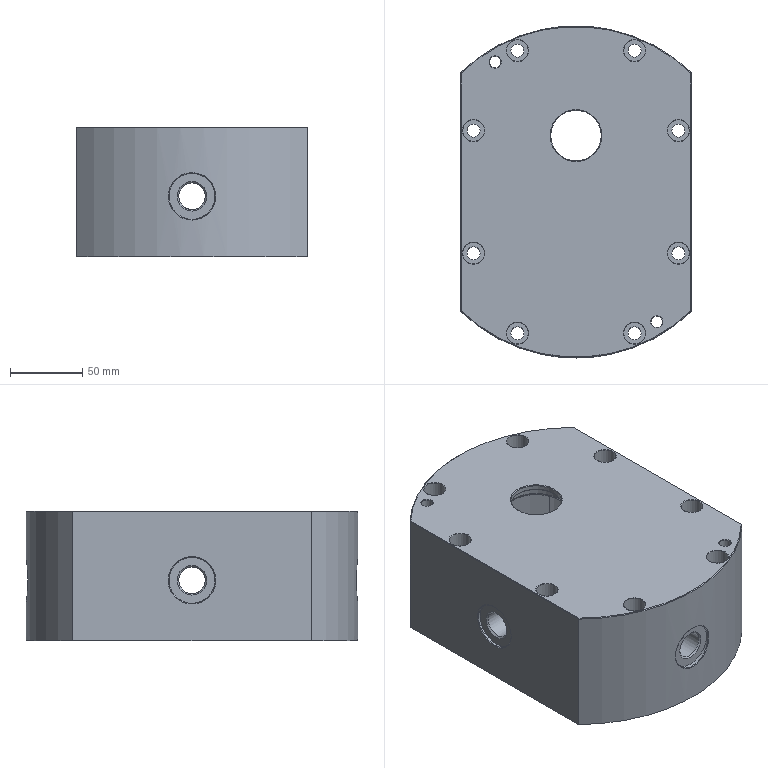NC program | NX | posted with a generic post | part box 160 x 230 x 90 mm
Lines 1 to 991 of 9223:
N10 G17 G21 G94 G90
(FLOOR_WALL_COPY_1 , TOOL : D50)
N12 T02 M6
N14 G54
N16 G17 G0 G90 X-153. Y89.997 B0. C0. S1200 M3
N18 G43 Z30. H2
N20 Z12.658
N22 G94 G1 Z9.658 F1000.
N24 X-150.
N26 X150. F2000.
N28 Y49.998
N30 X-150.
N32 Y9.999
N34 X150.
N36 Y-30.001
N38 X-150.
N40 Y-65.341
N42 Y-70.
N44 X150.
N46 X153.
N48 Z12.658
N50 G0 Z30.
N52 X-153. Y89.997
N54 Z12.317
N56 G1 Z9.317 F1000.
N58 X-150.
N60 X150. F2000.
N62 Y49.998
N64 X-150.
N66 Y9.999
N68 X150.
N70 Y-30.001
N72 X-150.
N74 Y-65.341
N76 Y-70.
N78 X150.
N80 X153.
N82 Z12.317
N84 G0 Z30.
N86 X-153. Y89.997
N88 Z11.976
N90 G1 Z8.976 F1000.
N92 X-150.
N94 X150. F2000.
N96 Y49.998
N98 X-150.
N100 Y9.999
N102 X150.
N104 Y-30.001
N106 X-150.
N108 Y-65.341
N110 Y-70.
N112 X150.
N114 X153.
N116 Z11.976
N118 G0 Z30.
N120 X-153. Y89.997
N122 Z11.634
N124 G1 Z8.634 F1000.
N126 X-150.
N128 X150. F2000.
N130 Y49.998
N132 X-150.
N134 Y9.999
N136 X150.
N138 Y-30.001
N140 X-150.
N142 Y-65.341
N144 Y-70.
N146 X150.
N148 X153.
N150 Z11.634
N152 G0 Z30.
N154 X-153. Y89.997
N156 Z11.293
N158 G1 Z8.293 F1000.
N160 X-150.
N162 X150. F2000.
N164 Y49.998
N166 X-150.
N168 Y9.999
N170 X150.
N172 Y-30.001
N174 X-150.
N176 Y-65.341
N178 Y-70.
N180 X150.
N182 X153.
N184 Z11.293
N186 G0 Z30.
N188 X-153. Y89.997
N190 Z10.951
N192 G1 Z7.951 F1000.
N194 X-150.
N196 X150. F2000.
N198 Y49.998
N200 X-150.
N202 Y9.999
N204 X150.
N206 Y-30.001
N208 X-150.
N210 Y-65.341
N212 Y-70.
N214 X150.
N216 X153.
N218 Z10.951
N220 G0 Z30.
N222 X-153. Y89.997
N224 Z10.61
N226 G1 Z7.61 F1000.
N228 X-150.
N230 X150. F2000.
N232 Y49.998
N234 X-150.
N236 Y9.999
N238 X150.
N240 Y-30.001
N242 X-150.
N244 Y-65.341
N246 Y-70.
N248 X150.
N250 X153.
N252 Z10.61
N254 G0 Z30.
N256 X-153. Y89.997
N258 Z10.269
N260 G1 Z7.269 F1000.
N262 X-150.
N264 X150. F2000.
N266 Y49.998
N268 X-150.
N270 Y9.999
N272 X150.
N274 Y-30.001
N276 X-150.
N278 Y-65.341
N280 Y-70.
N282 X150.
N284 X153.
N286 Z10.269
N288 G0 Z30.
N290 X-153. Y89.997
N292 Z9.927
N294 G1 Z6.927 F1000.
N296 X-150.
N298 X150. F2000.
N300 Y49.998
N302 X-150.
N304 Y9.999
N306 X150.
N308 Y-30.001
N310 X-150.
N312 Y-65.341
N314 Y-70.
N316 X150.
N318 X153.
N320 Z9.927
N322 G0 Z30.
N324 X-153. Y89.997
N326 Z9.586
N328 G1 Z6.586 F1000.
N330 X-150.
N332 X150. F2000.
N334 Y49.998
N336 X-150.
N338 Y9.999
N340 X150.
N342 Y-30.001
N344 X-150.
N346 Y-65.341
N348 Y-70.
N350 X150.
N352 X153.
N354 Z9.586
N356 G0 Z30.
N358 X-153. Y89.997
N360 Z9.245
N362 G1 Z6.245 F1000.
N364 X-150.
N366 X150. F2000.
N368 Y49.998
N370 X-150.
N372 Y9.999
N374 X150.
N376 Y-30.001
N378 X-150.
N380 Y-65.341
N382 Y-70.
N384 X150.
N386 X153.
N388 Z9.245
N390 G0 Z30.
N392 X-153. Y89.997
N394 Z8.903
N396 G1 Z5.903 F1000.
N398 X-150.
N400 X150. F2000.
N402 Y49.998
N404 X-150.
N406 Y9.999
N408 X150.
N410 Y-30.001
N412 X-150.
N414 Y-65.341
N416 Y-70.
N418 X150.
N420 X153.
N422 Z8.903
N424 G0 Z30.
N426 X-153. Y89.997
N428 Z8.562
N430 G1 Z5.562 F1000.
N432 X-150.
N434 X150. F2000.
N436 Y49.998
N438 X-150.
N440 Y9.999
N442 X150.
N444 Y-30.001
N446 X-150.
N448 Y-65.341
N450 Y-70.
N452 X150.
N454 X153.
N456 Z8.562
N458 G0 Z30.
N460 X-153. Y89.997
N462 Z8.221
N464 G1 Z5.221 F1000.
N466 X-150.
N468 X150. F2000.
N470 Y49.998
N472 X-150.
N474 Y9.999
N476 X150.
N478 Y-30.001
N480 X-150.
N482 Y-65.341
N484 Y-70.
N486 X150.
N488 X153.
N490 Z8.221
N492 G0 Z30.
N494 X-153. Y89.997
N496 Z7.879
N498 G1 Z4.879 F1000.
N500 X-150.
N502 X150. F2000.
N504 Y49.998
N506 X-150.
N508 Y9.999
N510 X150.
N512 Y-30.001
N514 X-150.
N516 Y-65.341
N518 Y-70.
N520 X150.
N522 X153.
N524 Z7.879
N526 G0 Z30.
N528 X-153. Y89.997
N530 Z7.538
N532 G1 Z4.538 F1000.
N534 X-150.
N536 X150. F2000.
N538 Y49.998
N540 X-150.
N542 Y9.999
N544 X150.
N546 Y-30.001
N548 X-150.
N550 Y-65.341
N552 Y-70.
N554 X150.
N556 X153.
N558 Z7.538
N560 G0 Z30.
N562 X-153. Y89.997
N564 Z7.196
N566 G1 Z4.196 F1000.
N568 X-150.
N570 X150. F2000.
N572 Y49.998
N574 X-150.
N576 Y9.999
N578 X150.
N580 Y-30.001
N582 X-150.
N584 Y-65.341
N586 Y-70.
N588 X150.
N590 X153.
N592 Z7.196
N594 G0 Z30.
N596 X-153. Y89.997
N598 Z6.855
N600 G1 Z3.855 F1000.
N602 X-150.
N604 X150. F2000.
N606 Y49.998
N608 X-150.
N610 Y9.999
N612 X150.
N614 Y-30.001
N616 X-150.
N618 Y-65.341
N620 Y-70.
N622 X150.
N624 X153.
N626 Z6.855
N628 G0 Z30.
N630 X-153. Y89.997
N632 Z6.514
N634 G1 Z3.514 F1000.
N636 X-150.
N638 X150. F2000.
N640 Y49.998
N642 X-150.
N644 Y9.999
N646 X150.
N648 Y-30.001
N650 X-150.
N652 Y-65.341
N654 Y-70.
N656 X150.
N658 X153.
N660 Z6.514
N662 G0 Z30.
N664 X-153. Y89.997
N666 Z6.172
N668 G1 Z3.172 F1000.
N670 X-150.
N672 X150. F2000.
N674 Y49.998
N676 X-150.
N678 Y9.999
N680 X150.
N682 Y-30.001
N684 X-150.
N686 Y-65.341
N688 Y-70.
N690 X150.
N692 X153.
N694 Z6.172
N696 G0 Z30.
N698 X-153. Y89.997
N700 Z5.831
N702 G1 Z2.831 F1000.
N704 X-150.
N706 X150. F2000.
N708 Y49.998
N710 X-150.
N712 Y9.999
N714 X150.
N716 Y-30.001
N718 X-150.
N720 Y-65.341
N722 Y-70.
N724 X150.
N726 X153.
N728 Z5.831
N730 G0 Z30.
N732 X-153. Y89.997
N734 Z5.49
N736 G1 Z2.49 F1000.
N738 X-150.
N740 X150. F2000.
N742 Y49.998
N744 X-150.
N746 Y9.999
N748 X150.
N750 Y-30.001
N752 X-150.
N754 Y-65.341
N756 Y-70.
N758 X150.
N760 X153.
N762 Z5.49
N764 G0 Z30.
N766 X-153. Y89.997
N768 Z5.148
N770 G1 Z2.148 F1000.
N772 X-150.
N774 X150. F2000.
N776 Y49.998
N778 X-150.
N780 Y9.999
N782 X150.
N784 Y-30.001
N786 X-150.
N788 Y-65.341
N790 Y-70.
N792 X150.
N794 X153.
N796 Z5.148
N798 G0 Z30.
N800 X-153. Y89.997
N802 Z4.807
N804 G1 Z1.807 F1000.
N806 X-150.
N808 X150. F2000.
N810 Y49.998
N812 X-150.
N814 Y9.999
N816 X150.
N818 Y-30.001
N820 X-150.
N822 Y-65.341
N824 Y-70.
N826 X150.
N828 X153.
N830 Z4.807
N832 G0 Z30.
N834 X-153. Y89.997
N836 Z4.465
N838 G1 Z1.465 F1000.
N840 X-150.
N842 X150. F2000.
N844 Y49.998
N846 X-150.
N848 Y9.999
N850 X150.
N852 Y-30.001
N854 X-150.
N856 Y-65.341
N858 Y-70.
N860 X150.
N862 X153.
N864 Z4.465
N866 G0 Z30.
N868 X-153. Y89.997
N870 Z4.124
N872 G1 Z1.124 F1000.
N874 X-150.
N876 X150. F2000.
N878 Y49.998
N880 X-150.
N882 Y9.999
N884 X150.
N886 Y-30.001
N888 X-150.
N890 Y-65.341
N892 Y-70.
N894 X150.
N896 X153.
N898 Z4.124
N900 G0 Z30.
N902 X-153. Y89.997
N904 Z3.783
N906 G1 Z0.783 F1000.
N908 X-150.
N910 X150. F2000.
N912 Y49.998
N914 X-150.
N916 Y9.999
N918 X150.
N920 Y-30.001
N922 X-150.
N924 Y-65.341
N926 Y-70.
N928 X150.
N930 X153.
N932 Z3.783
N934 G0 Z30.
N936 X-153. Y89.997
N938 Z3.441
N940 G1 Z0.441 F1000.
N942 X-150.
N944 X150. F2000.
N946 Y49.998
N948 X-150.
N950 Y9.999
N952 X150.
N954 Y-30.001
N956 X-150.
N958 Y-65.341
N960 Y-70.
N962 X150.
N964 X153.
N966 Z3.441
N968 G0 Z30.
N970 X-153. Y89.997
N972 Z3.1
N974 G1 Z0.1 F1000.
N976 X-150.
N978 X150. F2000.
N980 Y49.998
N982 X-150.
N984 Y9.999
N986 X150.
N988 Y-30.001
N990 X-150.
N992 Y-65.341
N994 Y-70.
N996 X150.
N998 X153.
N1000 Z3.1
N1002 G0 Z30.
(FLOOR_WALL_COPY_COPY , TOOL : D50)
N1004 X-153. Y89.997 S2500
N1006 Z3.
N1008 G1 Z0. F1000.
N1010 X-150.
N1012 X150.
N1014 Y49.998
N1016 X-150.
N1018 Y9.999
N1020 X150.
N1022 Y-30.001
N1024 X-150.
N1026 Y-65.341
N1028 Y-70.
N1030 X150.
N1032 X153.
N1034 Z3.
N1036 G0 Z30.
N1038 M5
(DRILLING_COPY_1 , TOOL : ZXZ)
N1040 T01 M6
N1042 G54
N1044 G17 G0 G90 X-42.5 Y71. B0. C0. S5000 M3
N1046 G43 Z30. H1
N1048 G94 G81 G98 Z-1. F250. R3.
N1050 X-90. Y56.
N1052 X-97.931 Y40.564
N1054 Y-40.564
N1056 X-42.5 Y-71.
N1058 X42.5
N1060 X90. Y-56.
N1062 X97.931 Y-40.564
N1064 Y40.564
N1066 X42.5 Y71.
N1068 G80
N1070 G0 X42.5 Y71. Z30.
N1072 M5
(DRILLING_COPY , TOOL : 9.0ZT)
N1074 T09 M6
N1076 G54
N1078 G17 G0 G90 X42.5 Y-71. B0. C0. S2000 M3
N1080 G43 Z30. H9
N1082 G94 G83 G98 Z-69.204 F150. Q2. R3.
N1084 X97.931 Y-40.564
N1086 Y40.564
N1088 X42.5 Y71.
N1090 X-42.5
N1092 X-97.931 Y40.564
N1094 Y-40.564
N1096 X-42.5 Y-71.
N1098 G80
N1100 G0 X-42.5 Y-71. Z30.
N1102 M5
(DRILLING_COPY_COPY , TOOL : 7.8ZT)
N1104 T08 M6
N1106 G54
N1108 G17 G0 G90 X-90. Y56. B0. C0. S2000 M3
N1110 G43 Z30. H8
N1112 G94 G83 G98 Z-23.343 F150. Q2. R3.
N1114 X90. Y-56.
N1116 G80
N1118 G0 X90. Y-56. Z30.
N1120 M5
(DRILLING_COPY_COPY_COPY , TOOL : 8.0JD)
N1122 T18 M6
N1124 G54
N1126 G17 G0 G90 X-90. Y56. B0. C0. S800 M3
N1128 G43 Z30. H18
N1130 G94 G85 G98 Z-20. F40. R3.
N1132 X90. Y-56.
N1134 G80
N1136 G0 X90. Y-56. Z30.
N1138 M5
(PLANAR_PROFILE , TOOL : D3)
N1140 T03 M6
N1142 G54
N1144 G17 G0 G90 X0. Y62.5 B0. C0. S5000 M3
N1146 G43 Z30. H3
N1148 Z3.
N1150 G94 G1 Z-0.05 F500.
N1152 X-65.077 F1100.
N1154 G3 X-81.346 Y53.75 R19.5
N1156 X-81.346 Y-53.75 R97.5
N1158 X-65.077 Y-62.5 R19.5
N1160 G1 X65.077
N1162 G3 X81.346 Y-53.75 R19.5
N1164 X81.346 Y53.75 R97.5
N1166 X65.077 Y62.5 R19.5
N1168 G1 X0.
N1170 Z2.95
N1172 Z-0.1 F500.
N1174 X65.077 F1100.
N1176 G2 X81.346 Y53.75 R19.5
N1178 X81.346 Y-53.75 R97.5
N1180 X65.077 Y-62.5 R19.5
N1182 G1 X-65.077
N1184 G2 X-81.346 Y-53.75 R19.5
N1186 X-81.346 Y53.75 R97.5
N1188 X-65.077 Y62.5 R19.5
N1190 G1 X0.
N1192 Z2.9
N1194 Z-0.15 F500.
N1196 X-65.077 F1100.
N1198 G3 X-81.346 Y53.75 R19.5
N1200 X-81.346 Y-53.75 R97.5
N1202 X-65.077 Y-62.5 R19.5
N1204 G1 X65.077
N1206 G3 X81.346 Y-53.75 R19.5
N1208 X81.346 Y53.75 R97.5
N1210 X65.077 Y62.5 R19.5
N1212 G1 X0.
N1214 Z2.85
N1216 Z-0.2 F500.
N1218 X65.077 F1100.
N1220 G2 X81.346 Y53.75 R19.5
N1222 X81.346 Y-53.75 R97.5
N1224 X65.077 Y-62.5 R19.5
N1226 G1 X-65.077
N1228 G2 X-81.346 Y-53.75 R19.5
N1230 X-81.346 Y53.75 R97.5
N1232 X-65.077 Y62.5 R19.5
N1234 G1 X0.
N1236 Z2.8
N1238 Z-0.25 F500.
N1240 X-65.077 F1100.
N1242 G3 X-81.346 Y53.75 R19.5
N1244 X-81.346 Y-53.75 R97.5
N1246 X-65.077 Y-62.5 R19.5
N1248 G1 X65.077
N1250 G3 X81.346 Y-53.75 R19.5
N1252 X81.346 Y53.75 R97.5
N1254 X65.077 Y62.5 R19.5
N1256 G1 X0.
N1258 Z2.75
N1260 Z-0.3 F500.
N1262 X65.077 F1100.
N1264 G2 X81.346 Y53.75 R19.5
N1266 X81.346 Y-53.75 R97.5
N1268 X65.077 Y-62.5 R19.5
N1270 G1 X-65.077
N1272 G2 X-81.346 Y-53.75 R19.5
N1274 X-81.346 Y53.75 R97.5
N1276 X-65.077 Y62.5 R19.5
N1278 G1 X0.
N1280 Z2.7
N1282 Z-0.35 F500.
N1284 X-65.077 F1100.
N1286 G3 X-81.346 Y53.75 R19.5
N1288 X-81.346 Y-53.75 R97.5
N1290 X-65.077 Y-62.5 R19.5
N1292 G1 X65.077
N1294 G3 X81.346 Y-53.75 R19.5
N1296 X81.346 Y53.75 R97.5
N1298 X65.077 Y62.5 R19.5
N1300 G1 X0.
N1302 Z2.65
N1304 Z-0.4 F500.
N1306 X65.077 F1100.
N1308 G2 X81.346 Y53.75 R19.5
N1310 X81.346 Y-53.75 R97.5
N1312 X65.077 Y-62.5 R19.5
N1314 G1 X-65.077
N1316 G2 X-81.346 Y-53.75 R19.5
N1318 X-81.346 Y53.75 R97.5
N1320 X-65.077 Y62.5 R19.5
N1322 G1 X0.
N1324 Z2.6
N1326 Z-0.45 F500.
N1328 X-65.077 F1100.
N1330 G3 X-81.346 Y53.75 R19.5
N1332 X-81.346 Y-53.75 R97.5
N1334 X-65.077 Y-62.5 R19.5
N1336 G1 X65.077
N1338 G3 X81.346 Y-53.75 R19.5
N1340 X81.346 Y53.75 R97.5
N1342 X65.077 Y62.5 R19.5
N1344 G1 X0.
N1346 Z2.55
N1348 Z-0.5 F500.
N1350 X65.077 F1100.
N1352 G2 X81.346 Y53.75 R19.5
N1354 X81.346 Y-53.75 R97.5
N1356 X65.077 Y-62.5 R19.5
N1358 G1 X-65.077
N1360 G2 X-81.346 Y-53.75 R19.5
N1362 X-81.346 Y53.75 R97.5
N1364 X-65.077 Y62.5 R19.5
N1366 G1 X0.
N1368 Z2.5
N1370 Z-0.55 F500.
N1372 X-65.077 F1100.
N1374 G3 X-81.346 Y53.75 R19.5
N1376 X-81.346 Y-53.75 R97.5
N1378 X-65.077 Y-62.5 R19.5
N1380 G1 X65.077
N1382 G3 X81.346 Y-53.75 R19.5
N1384 X81.346 Y53.75 R97.5
N1386 X65.077 Y62.5 R19.5
N1388 G1 X0.
N1390 Z2.45
N1392 Z-0.6 F500.
N1394 X65.077 F1100.
N1396 G2 X81.346 Y53.75 R19.5
N1398 X81.346 Y-53.75 R97.5
N1400 X65.077 Y-62.5 R19.5
N1402 G1 X-65.077
N1404 G2 X-81.346 Y-53.75 R19.5
N1406 X-81.346 Y53.75 R97.5
N1408 X-65.077 Y62.5 R19.5
N1410 G1 X0.
N1412 Z2.4
N1414 Z-0.65 F500.
N1416 X-65.077 F1100.
N1418 G3 X-81.346 Y53.75 R19.5
N1420 X-81.346 Y-53.75 R97.5
N1422 X-65.077 Y-62.5 R19.5
N1424 G1 X65.077
N1426 G3 X81.346 Y-53.75 R19.5
N1428 X81.346 Y53.75 R97.5
N1430 X65.077 Y62.5 R19.5
N1432 G1 X0.
N1434 Z2.35
N1436 Z-0.7 F500.
N1438 X65.077 F1100.
N1440 G2 X81.346 Y53.75 R19.5
N1442 X81.346 Y-53.75 R97.5
N1444 X65.077 Y-62.5 R19.5
N1446 G1 X-65.077
N1448 G2 X-81.346 Y-53.75 R19.5
N1450 X-81.346 Y53.75 R97.5
N1452 X-65.077 Y62.5 R19.5
N1454 G1 X0.
N1456 Z2.3
N1458 Z-0.75 F500.
N1460 X-65.077 F1100.
N1462 G3 X-81.346 Y53.75 R19.5
N1464 X-81.346 Y-53.75 R97.5
N1466 X-65.077 Y-62.5 R19.5
N1468 G1 X65.077
N1470 G3 X81.346 Y-53.75 R19.5
N1472 X81.346 Y53.75 R97.5
N1474 X65.077 Y62.5 R19.5
N1476 G1 X0.
N1478 Z2.25
N1480 Z-0.8 F500.
N1482 X65.077 F1100.
N1484 G2 X81.346 Y53.75 R19.5
N1486 X81.346 Y-53.75 R97.5
N1488 X65.077 Y-62.5 R19.5
N1490 G1 X-65.077
N1492 G2 X-81.346 Y-53.75 R19.5
N1494 X-81.346 Y53.75 R97.5
N1496 X-65.077 Y62.5 R19.5
N1498 G1 X0.
N1500 Z2.2
N1502 Z-0.85 F500.
N1504 X-65.077 F1100.
N1506 G3 X-81.346 Y53.75 R19.5
N1508 X-81.346 Y-53.75 R97.5
N1510 X-65.077 Y-62.5 R19.5
N1512 G1 X65.077
N1514 G3 X81.346 Y-53.75 R19.5
N1516 X81.346 Y53.75 R97.5
N1518 X65.077 Y62.5 R19.5
N1520 G1 X0.
N1522 Z2.15
N1524 Z-0.9 F500.
N1526 X65.077 F1100.
N1528 G2 X81.346 Y53.75 R19.5
N1530 X81.346 Y-53.75 R97.5
N1532 X65.077 Y-62.5 R19.5
N1534 G1 X-65.077
N1536 G2 X-81.346 Y-53.75 R19.5
N1538 X-81.346 Y53.75 R97.5
N1540 X-65.077 Y62.5 R19.5
N1542 G1 X0.
N1544 Z2.1
N1546 Z-0.95 F500.
N1548 X-65.077 F1100.
N1550 G3 X-81.346 Y53.75 R19.5
N1552 X-81.346 Y-53.75 R97.5
N1554 X-65.077 Y-62.5 R19.5
N1556 G1 X65.077
N1558 G3 X81.346 Y-53.75 R19.5
N1560 X81.346 Y53.75 R97.5
N1562 X65.077 Y62.5 R19.5
N1564 G1 X0.
N1566 Z2.05
N1568 Z-1. F500.
N1570 X65.077 F1100.
N1572 G2 X81.346 Y53.75 R19.5
N1574 X81.346 Y-53.75 R97.5
N1576 X65.077 Y-62.5 R19.5
N1578 G1 X-65.077
N1580 G2 X-81.346 Y-53.75 R19.5
N1582 X-81.346 Y53.75 R97.5
N1584 X-65.077 Y62.5 R19.5
N1586 G1 X0.
N1588 Z2.
N1590 Z-1.05 F500.
N1592 X-65.077 F1100.
N1594 G3 X-81.346 Y53.75 R19.5
N1596 X-81.346 Y-53.75 R97.5
N1598 X-65.077 Y-62.5 R19.5
N1600 G1 X65.077
N1602 G3 X81.346 Y-53.75 R19.5
N1604 X81.346 Y53.75 R97.5
N1606 X65.077 Y62.5 R19.5
N1608 G1 X0.
N1610 Z1.95
N1612 Z-1.1 F500.
N1614 X65.077 F1100.
N1616 G2 X81.346 Y53.75 R19.5
N1618 X81.346 Y-53.75 R97.5
N1620 X65.077 Y-62.5 R19.5
N1622 G1 X-65.077
N1624 G2 X-81.346 Y-53.75 R19.5
N1626 X-81.346 Y53.75 R97.5
N1628 X-65.077 Y62.5 R19.5
N1630 G1 X0.
N1632 Z1.9
N1634 Z-1.15 F500.
N1636 X-65.077 F1100.
N1638 G3 X-81.346 Y53.75 R19.5
N1640 X-81.346 Y-53.75 R97.5
N1642 X-65.077 Y-62.5 R19.5
N1644 G1 X65.077
N1646 G3 X81.346 Y-53.75 R19.5
N1648 X81.346 Y53.75 R97.5
N1650 X65.077 Y62.5 R19.5
N1652 G1 X0.
N1654 Z1.85
N1656 Z-1.2 F500.
N1658 X65.077 F1100.
N1660 G2 X81.346 Y53.75 R19.5
N1662 X81.346 Y-53.75 R97.5
N1664 X65.077 Y-62.5 R19.5
N1666 G1 X-65.077
N1668 G2 X-81.346 Y-53.75 R19.5
N1670 X-81.346 Y53.75 R97.5
N1672 X-65.077 Y62.5 R19.5
N1674 G1 X0.
N1676 Z1.8
N1678 Z-1.25 F500.
N1680 X-65.077 F1100.
N1682 G3 X-81.346 Y53.75 R19.5
N1684 X-81.346 Y-53.75 R97.5
N1686 X-65.077 Y-62.5 R19.5
N1688 G1 X65.077
N1690 G3 X81.346 Y-53.75 R19.5
N1692 X81.346 Y53.75 R97.5
N1694 X65.077 Y62.5 R19.5
N1696 G1 X0.
N1698 Z1.75
N1700 Z-1.3 F500.
N1702 X65.077 F1100.
N1704 G2 X81.346 Y53.75 R19.5
N1706 X81.346 Y-53.75 R97.5
N1708 X65.077 Y-62.5 R19.5
N1710 G1 X-65.077
N1712 G2 X-81.346 Y-53.75 R19.5
N1714 X-81.346 Y53.75 R97.5
N1716 X-65.077 Y62.5 R19.5
N1718 G1 X0.
N1720 Z1.7
N1722 Z-1.35 F500.
N1724 X-65.077 F1100.
N1726 G3 X-81.346 Y53.75 R19.5
N1728 X-81.346 Y-53.75 R97.5
N1730 X-65.077 Y-62.5 R19.5
N1732 G1 X65.077
N1734 G3 X81.346 Y-53.75 R19.5
N1736 X81.346 Y53.75 R97.5
N1738 X65.077 Y62.5 R19.5
N1740 G1 X0.
N1742 Z1.65
N1744 Z-1.4 F500.
N1746 X65.077 F1100.
N1748 G2 X81.346 Y53.75 R19.5
N1750 X81.346 Y-53.75 R97.5
N1752 X65.077 Y-62.5 R19.5
N1754 G1 X-65.077
N1756 G2 X-81.346 Y-53.75 R19.5
N1758 X-81.346 Y53.75 R97.5
N1760 X-65.077 Y62.5 R19.5
N1762 G1 X0.
N1764 Z1.6
N1766 Z-1.45 F500.
N1768 X-65.077 F1100.
N1770 G3 X-81.346 Y53.75 R19.5
N1772 X-81.346 Y-53.75 R97.5
N1774 X-65.077 Y-62.5 R19.5
N1776 G1 X65.077
N1778 G3 X81.346 Y-53.75 R19.5
N1780 X81.346 Y53.75 R97.5
N1782 X65.077 Y62.5 R19.5
N1784 G1 X0.
N1786 Z1.55
N1788 Z-1.5 F500.
N1790 X65.077 F1100.
N1792 G2 X81.346 Y53.75 R19.5
N1794 X81.346 Y-53.75 R97.5
N1796 X65.077 Y-62.5 R19.5
N1798 G1 X-65.077
N1800 G2 X-81.346 Y-53.75 R19.5
N1802 X-81.346 Y53.75 R97.5
N1804 X-65.077 Y62.5 R19.5
N1806 G1 X0.
N1808 Z1.5
N1810 Z-1.55 F500.
N1812 X-65.077 F1100.
N1814 G3 X-81.346 Y53.75 R19.5
N1816 X-81.346 Y-53.75 R97.5
N1818 X-65.077 Y-62.5 R19.5
N1820 G1 X65.077
N1822 G3 X81.346 Y-53.75 R19.5
N1824 X81.346 Y53.75 R97.5
N1826 X65.077 Y62.5 R19.5
N1828 G1 X0.
N1830 Z1.45
N1832 Z-1.6 F500.
N1834 X65.077 F1100.
N1836 G2 X81.346 Y53.75 R19.5
N1838 X81.346 Y-53.75 R97.5
N1840 X65.077 Y-62.5 R19.5
N1842 G1 X-65.077
N1844 G2 X-81.346 Y-53.75 R19.5
N1846 X-81.346 Y53.75 R97.5
N1848 X-65.077 Y62.5 R19.5
N1850 G1 X0.
N1852 Z1.4
N1854 Z-1.65 F500.
N1856 X-65.077 F1100.
N1858 G3 X-81.346 Y53.75 R19.5
N1860 X-81.346 Y-53.75 R97.5
N1862 X-65.077 Y-62.5 R19.5
N1864 G1 X65.077
N1866 G3 X81.346 Y-53.75 R19.5
N1868 X81.346 Y53.75 R97.5
N1870 X65.077 Y62.5 R19.5
N1872 G1 X0.
N1874 Z1.35
N1876 Z-1.7 F500.
N1878 X65.077 F1100.
N1880 G2 X81.346 Y53.75 R19.5
N1882 X81.346 Y-53.75 R97.5
N1884 X65.077 Y-62.5 R19.5
N1886 G1 X-65.077
N1888 G2 X-81.346 Y-53.75 R19.5
N1890 X-81.346 Y53.75 R97.5
N1892 X-65.077 Y62.5 R19.5
N1894 G1 X0.
N1896 Z1.3
N1898 Z-1.75 F500.
N1900 X-65.077 F1100.
N1902 G3 X-81.346 Y53.75 R19.5
N1904 X-81.346 Y-53.75 R97.5
N1906 X-65.077 Y-62.5 R19.5
N1908 G1 X65.077
N1910 G3 X81.346 Y-53.75 R19.5
N1912 X81.346 Y53.75 R97.5
N1914 X65.077 Y62.5 R19.5
N1916 G1 X0.
N1918 Z1.25
N1920 Z-1.8 F500.
N1922 X65.077 F1100.
N1924 G2 X81.346 Y53.75 R19.5
N1926 X81.346 Y-53.75 R97.5
N1928 X65.077 Y-62.5 R19.5
N1930 G1 X-65.077
N1932 G2 X-81.346 Y-53.75 R19.5
N1934 X-81.346 Y53.75 R97.5
N1936 X-65.077 Y62.5 R19.5
N1938 G1 X0.
N1940 Z1.2
N1942 G0 Z30.
N1944 M5